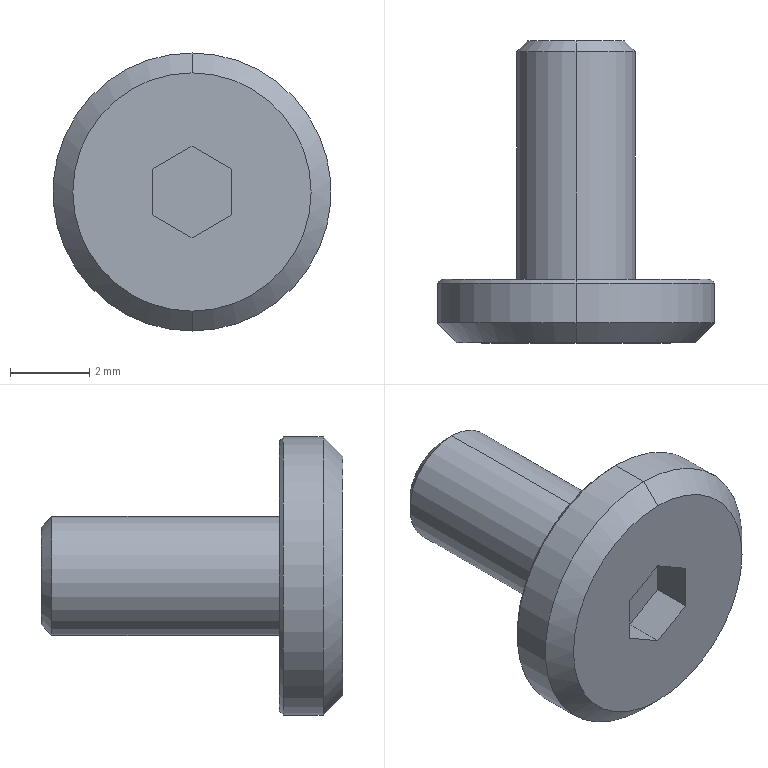Part | SolidWorks | features Chamfer 2, Extrusion 1, ICE 1, StudWizard 1 | 1 solid | 20 faces | box 7 x 7.6 x 7 mm | volume 97.472 mm3 | plane 10 | cone 6 | cylinder 4 | commonest cylinder face diameters 3 x2 7 x2
STEP:
#1=CARTESIAN_POINT('',(0.,1.6,3.4));
#2=VERTEX_POINT('',#1);
#3=CARTESIAN_POINT('',(0.,1.6,-3.4));
#4=VERTEX_POINT('',#3);
#5=CARTESIAN_POINT('',(0.,1.6,0.));
#6=DIRECTION('',(0.,1.,0.));
#7=DIRECTION('',(0.,0.,1.));
#8=AXIS2_PLACEMENT_3D('',#5,#6,#7);
#9=CIRCLE('',#8,3.4);
#10=EDGE_CURVE('',#2,#4,#9,.T.);
#11=ORIENTED_EDGE('',*,*,#10,.F.);
#12=CARTESIAN_POINT('',(0.,1.5,3.5));
#13=VERTEX_POINT('',#12);
#14=CARTESIAN_POINT('',(0.,1.6,3.4));
#15=DIRECTION('',(0.,-0.7071,0.7071));
#16=VECTOR('',#15,1000.);
#17=LINE('',#14,#16);
#18=EDGE_CURVE('',#2,#13,#17,.T.);
#19=ORIENTED_EDGE('',*,*,#18,.T.);
#20=CARTESIAN_POINT('',(0.,1.5,-3.5));
#21=VERTEX_POINT('',#20);
#22=CARTESIAN_POINT('',(0.,1.5,0.));
#23=DIRECTION('',(0.,-1.,0.));
#24=DIRECTION('',(0.,0.,1.));
#25=AXIS2_PLACEMENT_3D('',#22,#23,#24);
#26=CIRCLE('',#25,3.5);
#27=EDGE_CURVE('',#21,#13,#26,.T.);
#28=ORIENTED_EDGE('',*,*,#27,.F.);
#29=CARTESIAN_POINT('',(0.,1.6,-3.4));
#30=DIRECTION('',(0.,-0.7071,-0.7071));
#31=VECTOR('',#30,1000.);
#32=LINE('',#29,#31);
#33=EDGE_CURVE('',#4,#21,#32,.T.);
#34=ORIENTED_EDGE('',*,*,#33,.F.);
#35=EDGE_LOOP('',(#11,#19,#28,#34));
#36=FACE_OUTER_BOUND('',#35,.T.);
#37=CARTESIAN_POINT('',(0.,1.6,0.));
#38=DIRECTION('',(0.,-1.,0.));
#39=DIRECTION('',(0.,0.,-1.));
#40=AXIS2_PLACEMENT_3D('',#37,#38,#39);
#41=CONICAL_SURFACE('',#40,3.4,0.7854);
#42=ADVANCED_FACE('',(#36),#41,.T.);
#43=CARTESIAN_POINT('',(0.,0.,-3.));
#44=VERTEX_POINT('',#43);
#45=CARTESIAN_POINT('',(0.,0.,3.));
#46=VERTEX_POINT('',#45);
#47=CARTESIAN_POINT('',(0.,0.,0.));
#48=DIRECTION('',(0.,-1.,0.));
#49=DIRECTION('',(0.,0.,1.));
#50=AXIS2_PLACEMENT_3D('',#47,#48,#49);
#51=CIRCLE('',#50,3.);
#52=EDGE_CURVE('',#44,#46,#51,.T.);
#53=ORIENTED_EDGE('',*,*,#52,.F.);
#54=CARTESIAN_POINT('',(0.,0.5,-3.5));
#55=VERTEX_POINT('',#54);
#56=CARTESIAN_POINT('',(0.,0.5,-3.5));
#57=DIRECTION('',(0.,0.7071,-0.7071));
#58=VECTOR('',#57,1000.);
#59=LINE('',#56,#58);
#60=EDGE_CURVE('',#44,#55,#59,.T.);
#61=ORIENTED_EDGE('',*,*,#60,.T.);
#62=CARTESIAN_POINT('',(0.,0.5,3.5));
#63=VERTEX_POINT('',#62);
#64=CARTESIAN_POINT('',(0.,0.5,0.));
#65=DIRECTION('',(0.,1.,0.));
#66=DIRECTION('',(0.,0.,1.));
#67=AXIS2_PLACEMENT_3D('',#64,#65,#66);
#68=CIRCLE('',#67,3.5);
#69=EDGE_CURVE('',#63,#55,#68,.T.);
#70=ORIENTED_EDGE('',*,*,#69,.F.);
#71=CARTESIAN_POINT('',(0.,0.5,3.5));
#72=DIRECTION('',(0.,0.7071,0.7071));
#73=VECTOR('',#72,1000.);
#74=LINE('',#71,#73);
#75=EDGE_CURVE('',#46,#63,#74,.T.);
#76=ORIENTED_EDGE('',*,*,#75,.F.);
#77=EDGE_LOOP('',(#53,#61,#70,#76));
#78=FACE_OUTER_BOUND('',#77,.T.);
#79=CARTESIAN_POINT('',(0.,0.5,0.));
#80=DIRECTION('',(0.,1.,0.));
#81=DIRECTION('',(0.,0.,1.));
#82=AXIS2_PLACEMENT_3D('',#79,#80,#81);
#83=CONICAL_SURFACE('',#82,3.5,0.7854);
#84=ADVANCED_FACE('',(#78),#83,.T.);
#85=CARTESIAN_POINT('',(0.,7.33,-1.5));
#86=VERTEX_POINT('',#85);
#87=CARTESIAN_POINT('',(0.,7.33,1.5));
#88=VERTEX_POINT('',#87);
#89=CARTESIAN_POINT('',(0.,7.33,0.));
#90=DIRECTION('',(0.,-1.,0.));
#91=DIRECTION('',(0.,0.,-1.));
#92=AXIS2_PLACEMENT_3D('',#89,#90,#91);
#93=CIRCLE('',#92,1.5);
#94=EDGE_CURVE('',#86,#88,#93,.T.);
#95=ORIENTED_EDGE('',*,*,#94,.T.);
#96=CARTESIAN_POINT('',(0.,1.6,1.5));
#97=VERTEX_POINT('',#96);
#98=CARTESIAN_POINT('',(0.,1.6,1.5));
#99=DIRECTION('',(0.,-1.,0.));
#100=VECTOR('',#99,1000.);
#101=LINE('',#98,#100);
#102=EDGE_CURVE('',#88,#97,#101,.T.);
#103=ORIENTED_EDGE('',*,*,#102,.T.);
#104=CARTESIAN_POINT('',(0.,1.6,-1.5));
#105=VERTEX_POINT('',#104);
#106=CARTESIAN_POINT('',(0.,1.6,0.));
#107=DIRECTION('',(0.,-1.,0.));
#108=DIRECTION('',(0.,0.,-1.));
#109=AXIS2_PLACEMENT_3D('',#106,#107,#108);
#110=CIRCLE('',#109,1.5);
#111=EDGE_CURVE('',#105,#97,#110,.T.);
#112=ORIENTED_EDGE('',*,*,#111,.F.);
#113=CARTESIAN_POINT('',(0.,1.6,-1.5));
#114=DIRECTION('',(0.,-1.,0.));
#115=VECTOR('',#114,1000.);
#116=LINE('',#113,#115);
#117=EDGE_CURVE('',#86,#105,#116,.T.);
#118=ORIENTED_EDGE('',*,*,#117,.F.);
#119=EDGE_LOOP('',(#95,#103,#112,#118));
#120=FACE_OUTER_BOUND('',#119,.T.);
#121=CARTESIAN_POINT('',(0.,1.6,0.));
#122=DIRECTION('',(0.,-1.,0.));
#123=DIRECTION('',(0.,0.,-1.));
#124=AXIS2_PLACEMENT_3D('',#121,#122,#123);
#125=CYLINDRICAL_SURFACE('',#124,1.5);
#126=ADVANCED_FACE('',(#120),#125,.T.);
#127=CARTESIAN_POINT('',(0.,7.6,-1.23));
#128=VERTEX_POINT('',#127);
#129=CARTESIAN_POINT('',(0.,7.6,1.23));
#130=VERTEX_POINT('',#129);
#131=CARTESIAN_POINT('',(0.,7.6,0.));
#132=DIRECTION('',(0.,-1.,0.));
#133=DIRECTION('',(0.,0.,-1.));
#134=AXIS2_PLACEMENT_3D('',#131,#132,#133);
#135=CIRCLE('',#134,1.23);
#136=EDGE_CURVE('',#128,#130,#135,.T.);
#137=ORIENTED_EDGE('',*,*,#136,.T.);
#138=CARTESIAN_POINT('',(0.,7.33,1.5));
#139=DIRECTION('',(0.,-0.7071,0.7071));
#140=VECTOR('',#139,1000.);
#141=LINE('',#138,#140);
#142=EDGE_CURVE('',#130,#88,#141,.T.);
#143=ORIENTED_EDGE('',*,*,#142,.T.);
#144=ORIENTED_EDGE('',*,*,#94,.F.);
#145=CARTESIAN_POINT('',(0.,7.33,-1.5));
#146=DIRECTION('',(0.,-0.7071,-0.7071));
#147=VECTOR('',#146,1000.);
#148=LINE('',#145,#147);
#149=EDGE_CURVE('',#128,#86,#148,.T.);
#150=ORIENTED_EDGE('',*,*,#149,.F.);
#151=EDGE_LOOP('',(#137,#143,#144,#150));
#152=FACE_OUTER_BOUND('',#151,.T.);
#153=CARTESIAN_POINT('',(0.,7.33,0.));
#154=DIRECTION('',(0.,-1.,0.));
#155=DIRECTION('',(0.,0.,-1.));
#156=AXIS2_PLACEMENT_3D('',#153,#154,#155);
#157=CONICAL_SURFACE('',#156,1.5,0.7854);
#158=ADVANCED_FACE('',(#152),#157,.T.);
#159=ORIENTED_EDGE('',*,*,#27,.T.);
#160=CARTESIAN_POINT('',(0.,1.6,3.5));
#161=DIRECTION('',(0.,-1.,0.));
#162=VECTOR('',#161,1000.);
#163=LINE('',#160,#162);
#164=EDGE_CURVE('',#13,#63,#163,.T.);
#165=ORIENTED_EDGE('',*,*,#164,.T.);
#166=ORIENTED_EDGE('',*,*,#69,.T.);
#167=CARTESIAN_POINT('',(0.,1.6,-3.5));
#168=DIRECTION('',(0.,-1.,0.));
#169=VECTOR('',#168,1000.);
#170=LINE('',#167,#169);
#171=EDGE_CURVE('',#21,#55,#170,.T.);
#172=ORIENTED_EDGE('',*,*,#171,.F.);
#173=EDGE_LOOP('',(#159,#165,#166,#172));
#174=FACE_OUTER_BOUND('',#173,.T.);
#175=CARTESIAN_POINT('',(0.,1.6,0.));
#176=DIRECTION('',(0.,-1.,0.));
#177=DIRECTION('',(0.,0.,-1.));
#178=AXIS2_PLACEMENT_3D('',#175,#176,#177);
#179=CYLINDRICAL_SURFACE('',#178,3.5);
#180=ADVANCED_FACE('',(#174),#179,.T.);
#181=ORIENTED_EDGE('',*,*,#164,.F.);
#182=CARTESIAN_POINT('',(0.,1.5,0.));
#183=DIRECTION('',(0.,-1.,0.));
#184=DIRECTION('',(0.,0.,1.));
#185=AXIS2_PLACEMENT_3D('',#182,#183,#184);
#186=CIRCLE('',#185,3.5);
#187=EDGE_CURVE('',#13,#21,#186,.T.);
#188=ORIENTED_EDGE('',*,*,#187,.T.);
#189=ORIENTED_EDGE('',*,*,#171,.T.);
#190=CARTESIAN_POINT('',(0.,0.5,0.));
#191=DIRECTION('',(0.,1.,0.));
#192=DIRECTION('',(0.,0.,1.));
#193=AXIS2_PLACEMENT_3D('',#190,#191,#192);
#194=CIRCLE('',#193,3.5);
#195=EDGE_CURVE('',#55,#63,#194,.T.);
#196=ORIENTED_EDGE('',*,*,#195,.T.);
#197=EDGE_LOOP('',(#181,#188,#189,#196));
#198=FACE_OUTER_BOUND('',#197,.T.);
#199=CARTESIAN_POINT('',(0.,1.6,0.));
#200=DIRECTION('',(0.,-1.,0.));
#201=DIRECTION('',(0.,0.,-1.));
#202=AXIS2_PLACEMENT_3D('',#199,#200,#201);
#203=CYLINDRICAL_SURFACE('',#202,3.5);
#204=ADVANCED_FACE('',(#198),#203,.T.);
#205=CARTESIAN_POINT('',(0.,1.6,0.));
#206=DIRECTION('',(0.,1.,0.));
#207=DIRECTION('',(0.,0.,1.));
#208=AXIS2_PLACEMENT_3D('',#205,#206,#207);
#209=CIRCLE('',#208,3.4);
#210=EDGE_CURVE('',#4,#2,#209,.T.);
#211=ORIENTED_EDGE('',*,*,#210,.T.);
#212=ORIENTED_EDGE('',*,*,#10,.T.);
#213=EDGE_LOOP('',(#211,#212));
#214=FACE_OUTER_BOUND('',#213,.T.);
#215=ORIENTED_EDGE('',*,*,#111,.T.);
#216=CARTESIAN_POINT('',(0.,1.6,0.));
#217=DIRECTION('',(0.,-1.,0.));
#218=DIRECTION('',(0.,0.,-1.));
#219=AXIS2_PLACEMENT_3D('',#216,#217,#218);
#220=CIRCLE('',#219,1.5);
#221=EDGE_CURVE('',#97,#105,#220,.T.);
#222=ORIENTED_EDGE('',*,*,#221,.T.);
#223=EDGE_LOOP('',(#215,#222));
#224=FACE_BOUND('',#223,.T.);
#225=CARTESIAN_POINT('',(0.,1.6,0.));
#226=DIRECTION('',(0.,1.,0.));
#227=DIRECTION('',(0.,0.,1.));
#228=AXIS2_PLACEMENT_3D('',#225,#226,#227);
#229=PLANE('',#228);
#230=ADVANCED_FACE('',(#214,#224),#229,.T.);
#231=CARTESIAN_POINT('',(0.,0.,0.));
#232=DIRECTION('',(0.,-1.,0.));
#233=DIRECTION('',(0.,0.,1.));
#234=AXIS2_PLACEMENT_3D('',#231,#232,#233);
#235=CIRCLE('',#234,3.);
#236=EDGE_CURVE('',#46,#44,#235,.T.);
#237=ORIENTED_EDGE('',*,*,#236,.T.);
#238=ORIENTED_EDGE('',*,*,#52,.T.);
#239=EDGE_LOOP('',(#237,#238));
#240=FACE_OUTER_BOUND('',#239,.T.);
#241=CARTESIAN_POINT('',(0.,0.,1.155));
#242=VERTEX_POINT('',#241);
#243=CARTESIAN_POINT('',(-1.,0.,0.5774));
#244=VERTEX_POINT('',#243);
#245=CARTESIAN_POINT('',(0.,0.,1.155));
#246=DIRECTION('',(-0.866,0.,-0.5));
#247=VECTOR('',#246,1000.);
#248=LINE('',#245,#247);
#249=EDGE_CURVE('',#242,#244,#248,.T.);
#250=ORIENTED_EDGE('',*,*,#249,.F.);
#251=CARTESIAN_POINT('',(1.,0.,0.5774));
#252=VERTEX_POINT('',#251);
#253=CARTESIAN_POINT('',(1.,0.,0.5774));
#254=DIRECTION('',(-0.866,0.,0.5));
#255=VECTOR('',#254,1000.);
#256=LINE('',#253,#255);
#257=EDGE_CURVE('',#252,#242,#256,.T.);
#258=ORIENTED_EDGE('',*,*,#257,.F.);
#259=CARTESIAN_POINT('',(1.,0.,-0.5774));
#260=VERTEX_POINT('',#259);
#261=CARTESIAN_POINT('',(1.,0.,-0.5774));
#262=DIRECTION('',(0.,0.,1.));
#263=VECTOR('',#262,1000.);
#264=LINE('',#261,#263);
#265=EDGE_CURVE('',#260,#252,#264,.T.);
#266=ORIENTED_EDGE('',*,*,#265,.F.);
#267=CARTESIAN_POINT('',(0.,0.,-1.155));
#268=VERTEX_POINT('',#267);
#269=CARTESIAN_POINT('',(0.,0.,-1.155));
#270=DIRECTION('',(0.866,0.,0.5));
#271=VECTOR('',#270,1000.);
#272=LINE('',#269,#271);
#273=EDGE_CURVE('',#268,#260,#272,.T.);
#274=ORIENTED_EDGE('',*,*,#273,.F.);
#275=CARTESIAN_POINT('',(-1.,0.,-0.5774));
#276=VERTEX_POINT('',#275);
#277=CARTESIAN_POINT('',(-1.,0.,-0.5774));
#278=DIRECTION('',(0.866,0.,-0.5));
#279=VECTOR('',#278,1000.);
#280=LINE('',#277,#279);
#281=EDGE_CURVE('',#276,#268,#280,.T.);
#282=ORIENTED_EDGE('',*,*,#281,.F.);
#283=CARTESIAN_POINT('',(-1.,0.,0.5774));
#284=DIRECTION('',(0.,0.,-1.));
#285=VECTOR('',#284,1000.);
#286=LINE('',#283,#285);
#287=EDGE_CURVE('',#244,#276,#286,.T.);
#288=ORIENTED_EDGE('',*,*,#287,.F.);
#289=EDGE_LOOP('',(#250,#258,#266,#274,#282,#288));
#290=FACE_BOUND('',#289,.T.);
#291=CARTESIAN_POINT('',(0.,0.,0.));
#292=DIRECTION('',(0.,1.,0.));
#293=DIRECTION('',(0.,0.,1.));
#294=AXIS2_PLACEMENT_3D('',#291,#292,#293);
#295=PLANE('',#294);
#296=ADVANCED_FACE('',(#240,#290),#295,.F.);
#297=ORIENTED_EDGE('',*,*,#136,.F.);
#298=CARTESIAN_POINT('',(0.,7.6,0.));
#299=DIRECTION('',(0.,-1.,0.));
#300=DIRECTION('',(0.,0.,-1.));
#301=AXIS2_PLACEMENT_3D('',#298,#299,#300);
#302=CIRCLE('',#301,1.23);
#303=EDGE_CURVE('',#130,#128,#302,.T.);
#304=ORIENTED_EDGE('',*,*,#303,.F.);
#305=EDGE_LOOP('',(#297,#304));
#306=FACE_OUTER_BOUND('',#305,.T.);
#307=CARTESIAN_POINT('',(1.23,7.6,0.));
#308=DIRECTION('',(0.,1.,0.));
#309=DIRECTION('',(0.,0.,1.));
#310=AXIS2_PLACEMENT_3D('',#307,#308,#309);
#311=PLANE('',#310);
#312=ADVANCED_FACE('',(#306),#311,.T.);
#313=ORIENTED_EDGE('',*,*,#142,.F.);
#314=ORIENTED_EDGE('',*,*,#303,.T.);
#315=ORIENTED_EDGE('',*,*,#149,.T.);
#316=CARTESIAN_POINT('',(0.,7.33,0.));
#317=DIRECTION('',(0.,-1.,0.));
#318=DIRECTION('',(0.,0.,-1.));
#319=AXIS2_PLACEMENT_3D('',#316,#317,#318);
#320=CIRCLE('',#319,1.5);
#321=EDGE_CURVE('',#88,#86,#320,.T.);
#322=ORIENTED_EDGE('',*,*,#321,.F.);
#323=EDGE_LOOP('',(#313,#314,#315,#322));
#324=FACE_OUTER_BOUND('',#323,.T.);
#325=CARTESIAN_POINT('',(0.,7.33,0.));
#326=DIRECTION('',(0.,-1.,0.));
#327=DIRECTION('',(0.,0.,-1.));
#328=AXIS2_PLACEMENT_3D('',#325,#326,#327);
#329=CONICAL_SURFACE('',#328,1.5,0.7854);
#330=ADVANCED_FACE('',(#324),#329,.T.);
#331=ORIENTED_EDGE('',*,*,#102,.F.);
#332=ORIENTED_EDGE('',*,*,#321,.T.);
#333=ORIENTED_EDGE('',*,*,#117,.T.);
#334=ORIENTED_EDGE('',*,*,#221,.F.);
#335=EDGE_LOOP('',(#331,#332,#333,#334));
#336=FACE_OUTER_BOUND('',#335,.T.);
#337=CARTESIAN_POINT('',(0.,1.6,0.));
#338=DIRECTION('',(0.,-1.,0.));
#339=DIRECTION('',(0.,0.,-1.));
#340=AXIS2_PLACEMENT_3D('',#337,#338,#339);
#341=CYLINDRICAL_SURFACE('',#340,1.5);
#342=ADVANCED_FACE('',(#336),#341,.T.);
#343=ORIENTED_EDGE('',*,*,#257,.T.);
#344=CARTESIAN_POINT('',(0.,1.,1.155));
#345=VERTEX_POINT('',#344);
#346=CARTESIAN_POINT('',(0.,1.,1.155));
#347=DIRECTION('',(0.,-1.,0.));
#348=VECTOR('',#347,1000.);
#349=LINE('',#346,#348);
#350=EDGE_CURVE('',#345,#242,#349,.T.);
#351=ORIENTED_EDGE('',*,*,#350,.F.);
#352=CARTESIAN_POINT('',(1.,1.,0.5774));
#353=VERTEX_POINT('',#352);
#354=CARTESIAN_POINT('',(1.,1.,0.5774));
#355=DIRECTION('',(-0.866,0.,0.5));
#356=VECTOR('',#355,1000.);
#357=LINE('',#354,#356);
#358=EDGE_CURVE('',#353,#345,#357,.T.);
#359=ORIENTED_EDGE('',*,*,#358,.F.);
#360=CARTESIAN_POINT('',(1.,1.,0.5774));
#361=DIRECTION('',(0.,-1.,0.));
#362=VECTOR('',#361,1000.);
#363=LINE('',#360,#362);
#364=EDGE_CURVE('',#353,#252,#363,.T.);
#365=ORIENTED_EDGE('',*,*,#364,.T.);
#366=EDGE_LOOP('',(#343,#351,#359,#365));
#367=FACE_OUTER_BOUND('',#366,.T.);
#368=CARTESIAN_POINT('',(1.,1.,0.5774));
#369=DIRECTION('',(0.5,0.,0.866));
#370=DIRECTION('',(0.866,0.,-0.5));
#371=AXIS2_PLACEMENT_3D('',#368,#369,#370);
#372=PLANE('',#371);
#373=ADVANCED_FACE('',(#367),#372,.F.);
#374=ORIENTED_EDGE('',*,*,#265,.T.);
#375=ORIENTED_EDGE('',*,*,#364,.F.);
#376=CARTESIAN_POINT('',(1.,1.,-0.5774));
#377=VERTEX_POINT('',#376);
#378=CARTESIAN_POINT('',(1.,1.,-0.5774));
#379=DIRECTION('',(0.,0.,1.));
#380=VECTOR('',#379,1000.);
#381=LINE('',#378,#380);
#382=EDGE_CURVE('',#377,#353,#381,.T.);
#383=ORIENTED_EDGE('',*,*,#382,.F.);
#384=CARTESIAN_POINT('',(1.,1.,-0.5774));
#385=DIRECTION('',(0.,-1.,0.));
#386=VECTOR('',#385,1000.);
#387=LINE('',#384,#386);
#388=EDGE_CURVE('',#377,#260,#387,.T.);
#389=ORIENTED_EDGE('',*,*,#388,.T.);
#390=EDGE_LOOP('',(#374,#375,#383,#389));
#391=FACE_OUTER_BOUND('',#390,.T.);
#392=CARTESIAN_POINT('',(1.,1.,-0.5774));
#393=DIRECTION('',(1.,0.,0.));
#394=DIRECTION('',(0.,0.,-1.));
#395=AXIS2_PLACEMENT_3D('',#392,#393,#394);
#396=PLANE('',#395);
#397=ADVANCED_FACE('',(#391),#396,.F.);
#398=ORIENTED_EDGE('',*,*,#273,.T.);
#399=ORIENTED_EDGE('',*,*,#388,.F.);
#400=CARTESIAN_POINT('',(0.,1.,-1.155));
#401=VERTEX_POINT('',#400);
#402=CARTESIAN_POINT('',(0.,1.,-1.155));
#403=DIRECTION('',(0.866,0.,0.5));
#404=VECTOR('',#403,1000.);
#405=LINE('',#402,#404);
#406=EDGE_CURVE('',#401,#377,#405,.T.);
#407=ORIENTED_EDGE('',*,*,#406,.F.);
#408=CARTESIAN_POINT('',(0.,1.,-1.155));
#409=DIRECTION('',(0.,-1.,0.));
#410=VECTOR('',#409,1000.);
#411=LINE('',#408,#410);
#412=EDGE_CURVE('',#401,#268,#411,.T.);
#413=ORIENTED_EDGE('',*,*,#412,.T.);
#414=EDGE_LOOP('',(#398,#399,#407,#413));
#415=FACE_OUTER_BOUND('',#414,.T.);
#416=CARTESIAN_POINT('',(0.,1.,-1.155));
#417=DIRECTION('',(0.5,0.,-0.866));
#418=DIRECTION('',(-0.866,0.,-0.5));
#419=AXIS2_PLACEMENT_3D('',#416,#417,#418);
#420=PLANE('',#419);
#421=ADVANCED_FACE('',(#415),#420,.F.);
#422=ORIENTED_EDGE('',*,*,#281,.T.);
#423=ORIENTED_EDGE('',*,*,#412,.F.);
#424=CARTESIAN_POINT('',(-1.,1.,-0.5774));
#425=VERTEX_POINT('',#424);
#426=CARTESIAN_POINT('',(-1.,1.,-0.5774));
#427=DIRECTION('',(0.866,0.,-0.5));
#428=VECTOR('',#427,1000.);
#429=LINE('',#426,#428);
#430=EDGE_CURVE('',#425,#401,#429,.T.);
#431=ORIENTED_EDGE('',*,*,#430,.F.);
#432=CARTESIAN_POINT('',(-1.,1.,-0.5774));
#433=DIRECTION('',(0.,-1.,0.));
#434=VECTOR('',#433,1000.);
#435=LINE('',#432,#434);
#436=EDGE_CURVE('',#425,#276,#435,.T.);
#437=ORIENTED_EDGE('',*,*,#436,.T.);
#438=EDGE_LOOP('',(#422,#423,#431,#437));
#439=FACE_OUTER_BOUND('',#438,.T.);
#440=CARTESIAN_POINT('',(-1.,1.,-0.5774));
#441=DIRECTION('',(-0.5,0.,-0.866));
#442=DIRECTION('',(-0.866,0.,0.5));
#443=AXIS2_PLACEMENT_3D('',#440,#441,#442);
#444=PLANE('',#443);
#445=ADVANCED_FACE('',(#439),#444,.F.);
#446=ORIENTED_EDGE('',*,*,#287,.T.);
#447=ORIENTED_EDGE('',*,*,#436,.F.);
#448=CARTESIAN_POINT('',(-1.,1.,0.5774));
#449=VERTEX_POINT('',#448);
#450=CARTESIAN_POINT('',(-1.,1.,0.5774));
#451=DIRECTION('',(0.,0.,-1.));
#452=VECTOR('',#451,1000.);
#453=LINE('',#450,#452);
#454=EDGE_CURVE('',#449,#425,#453,.T.);
#455=ORIENTED_EDGE('',*,*,#454,.F.);
#456=CARTESIAN_POINT('',(-1.,1.,0.5774));
#457=DIRECTION('',(0.,-1.,0.));
#458=VECTOR('',#457,1000.);
#459=LINE('',#456,#458);
#460=EDGE_CURVE('',#449,#244,#459,.T.);
#461=ORIENTED_EDGE('',*,*,#460,.T.);
#462=EDGE_LOOP('',(#446,#447,#455,#461));
#463=FACE_OUTER_BOUND('',#462,.T.);
#464=CARTESIAN_POINT('',(-1.,1.,0.5774));
#465=DIRECTION('',(-1.,0.,0.));
#466=DIRECTION('',(0.,0.,1.));
#467=AXIS2_PLACEMENT_3D('',#464,#465,#466);
#468=PLANE('',#467);
#469=ADVANCED_FACE('',(#463),#468,.F.);
#470=ORIENTED_EDGE('',*,*,#249,.T.);
#471=ORIENTED_EDGE('',*,*,#460,.F.);
#472=CARTESIAN_POINT('',(0.,1.,1.155));
#473=DIRECTION('',(-0.866,0.,-0.5));
#474=VECTOR('',#473,1000.);
#475=LINE('',#472,#474);
#476=EDGE_CURVE('',#345,#449,#475,.T.);
#477=ORIENTED_EDGE('',*,*,#476,.F.);
#478=ORIENTED_EDGE('',*,*,#350,.T.);
#479=EDGE_LOOP('',(#470,#471,#477,#478));
#480=FACE_OUTER_BOUND('',#479,.T.);
#481=CARTESIAN_POINT('',(0.,1.,1.155));
#482=DIRECTION('',(-0.5,0.,0.866));
#483=DIRECTION('',(0.866,0.,0.5));
#484=AXIS2_PLACEMENT_3D('',#481,#482,#483);
#485=PLANE('',#484);
#486=ADVANCED_FACE('',(#480),#485,.F.);
#487=ORIENTED_EDGE('',*,*,#358,.T.);
#488=ORIENTED_EDGE('',*,*,#476,.T.);
#489=ORIENTED_EDGE('',*,*,#454,.T.);
#490=ORIENTED_EDGE('',*,*,#430,.T.);
#491=ORIENTED_EDGE('',*,*,#406,.T.);
#492=ORIENTED_EDGE('',*,*,#382,.T.);
#493=EDGE_LOOP('',(#487,#488,#489,#490,#491,#492));
#494=FACE_OUTER_BOUND('',#493,.T.);
#495=CARTESIAN_POINT('',(0.,1.,0.));
#496=DIRECTION('',(0.,-1.,0.));
#497=DIRECTION('',(0.,0.,-1.));
#498=AXIS2_PLACEMENT_3D('',#495,#496,#497);
#499=PLANE('',#498);
#500=ADVANCED_FACE('',(#494),#499,.T.);
#501=ORIENTED_EDGE('',*,*,#60,.F.);
#502=ORIENTED_EDGE('',*,*,#236,.F.);
#503=ORIENTED_EDGE('',*,*,#75,.T.);
#504=ORIENTED_EDGE('',*,*,#195,.F.);
#505=EDGE_LOOP('',(#501,#502,#503,#504));
#506=FACE_OUTER_BOUND('',#505,.T.);
#507=CARTESIAN_POINT('',(0.,0.5,0.));
#508=DIRECTION('',(0.,1.,0.));
#509=DIRECTION('',(0.,0.,1.));
#510=AXIS2_PLACEMENT_3D('',#507,#508,#509);
#511=CONICAL_SURFACE('',#510,3.5,0.7854);
#512=ADVANCED_FACE('',(#506),#511,.T.);
#513=ORIENTED_EDGE('',*,*,#18,.F.);
#514=ORIENTED_EDGE('',*,*,#210,.F.);
#515=ORIENTED_EDGE('',*,*,#33,.T.);
#516=ORIENTED_EDGE('',*,*,#187,.F.);
#517=EDGE_LOOP('',(#513,#514,#515,#516));
#518=FACE_OUTER_BOUND('',#517,.T.);
#519=CARTESIAN_POINT('',(0.,1.6,0.));
#520=DIRECTION('',(0.,-1.,0.));
#521=DIRECTION('',(0.,0.,-1.));
#522=AXIS2_PLACEMENT_3D('',#519,#520,#521);
#523=CONICAL_SURFACE('',#522,3.4,0.7854);
#524=ADVANCED_FACE('',(#518),#523,.T.);
#525=CLOSED_SHELL('',(#42,#84,#126,#158,#180,#204,#230,#296,#312,#330,#342,#373,#397,#421,#445,#469,#486,#500,#512,#524));
#526=MANIFOLD_SOLID_BREP('',#525);
#527=CARTESIAN_POINT('',(0.,0.,0.));
#528=DIRECTION('',(0.,0.,1.));
#529=DIRECTION('',(1.,0.,0.));
#530=AXIS2_PLACEMENT_3D('',#527,#528,#529);
#531=(LENGTH_UNIT()NAMED_UNIT(*)SI_UNIT(.MILLI.,.METRE.));
#532=UNCERTAINTY_MEASURE_WITH_UNIT(LENGTH_MEASURE(0.00001),#531,'','');
#533=(NAMED_UNIT(*)PLANE_ANGLE_UNIT()SI_UNIT($,.RADIAN.));
#534=(NAMED_UNIT(*)SI_UNIT($,.STERADIAN.)SOLID_ANGLE_UNIT());
#535=(GEOMETRIC_REPRESENTATION_CONTEXT(3)GLOBAL_UNCERTAINTY_ASSIGNED_CONTEXT((#532))GLOBAL_UNIT_ASSIGNED_CONTEXT((#531,#533,#534))REPRESENTATION_CONTEXT('',''));
#536=ADVANCED_BREP_SHAPE_REPRESENTATION('',(#526,#530),#535);